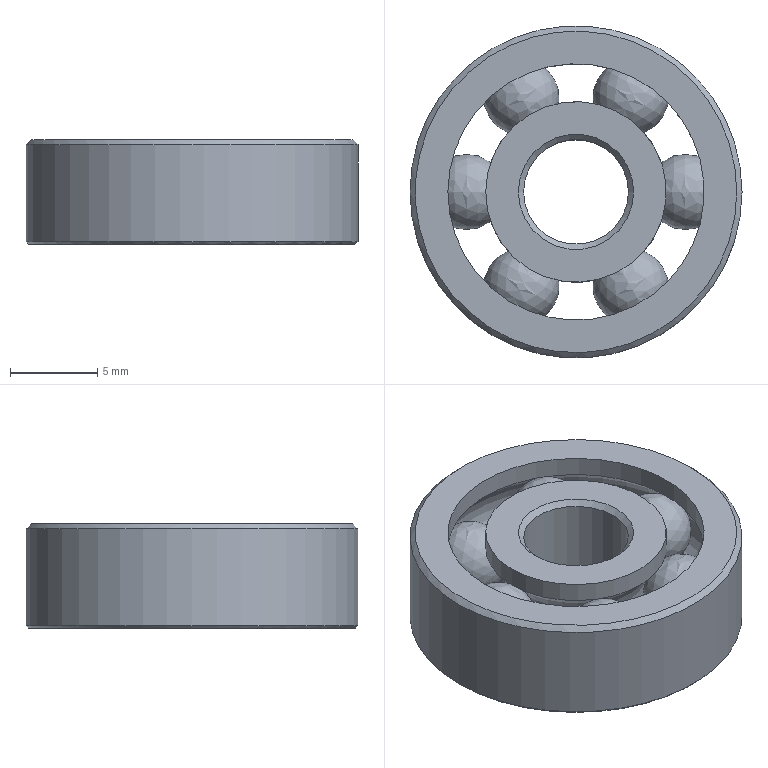Part | NX | features SWP104 11, INSTANCE_SET 5, CHAMFER 3, SKETCH 3, DATUM_CSYS 2, FSET 2, CIRCULAR_PATTERN 1, LINE 1 | 8 solids | 22 faces | box 19 x 19 x 6 mm | volume 1034 mm3 | sphere 6 | cylinder 5 | cone 5 | plane 4 | torus 2 | commonest cylinder face diameters 10.334 x2 6 x1 14.666 x1 19 x1
STEP:
#1=CARTESIAN_POINT('',(-2.042,-3.537,3.));
#2=VERTEX_POINT('',#1);
#3=VERTEX_LOOP('',#2);
#4=FACE_BOUND('',#3,.T.);
#5=CARTESIAN_POINT('',(-3.125,-5.413,3.));
#6=DIRECTION('',(-0.5,-0.866,0.));
#7=DIRECTION('',(0.,0.,1.));
#8=AXIS2_PLACEMENT_3D('',#5,#6,#7);
#9=SPHERICAL_SURFACE('',#8,2.166);
#10=ADVANCED_FACE('',(#4),#9,.T.);
#11=CLOSED_SHELL('',(#10));
#12=MANIFOLD_SOLID_BREP('',#11);
#13=CARTESIAN_POINT('',(5.167,0.,1.124));
#14=VERTEX_POINT('',#13);
#15=CARTESIAN_POINT('',(0.,0.,1.124));
#16=DIRECTION('',(0.,0.,1.));
#17=DIRECTION('',(1.,0.,0.));
#18=AXIS2_PLACEMENT_3D('',#15,#16,#17);
#19=CIRCLE('',#18,5.167);
#20=EDGE_CURVE('',#14,#14,#19,.T.);
#21=ORIENTED_EDGE('',*,*,#20,.F.);
#22=EDGE_LOOP('',(#21));
#23=FACE_BOUND('',#22,.T.);
#24=CARTESIAN_POINT('',(-5.167,0.,0.));
#25=VERTEX_POINT('',#24);
#26=CARTESIAN_POINT('',(0.,0.,0.));
#27=DIRECTION('',(0.,0.,-1.));
#28=DIRECTION('',(-1.,0.,0.));
#29=AXIS2_PLACEMENT_3D('',#26,#27,#28);
#30=CIRCLE('',#29,5.167);
#31=EDGE_CURVE('',#25,#25,#30,.T.);
#32=ORIENTED_EDGE('',*,*,#31,.F.);
#33=EDGE_LOOP('',(#32));
#34=FACE_BOUND('',#33,.T.);
#35=CARTESIAN_POINT('',(0.,0.,0.));
#36=DIRECTION('',(0.,0.,-1.));
#37=DIRECTION('',(-1.,0.,0.));
#38=AXIS2_PLACEMENT_3D('',#35,#36,#37);
#39=CYLINDRICAL_SURFACE('',#38,5.167);
#40=ADVANCED_FACE('',(#23,#34),#39,.T.);
#41=CARTESIAN_POINT('',(-3.,0.,0.3));
#42=VERTEX_POINT('',#41);
#43=CARTESIAN_POINT('',(0.,0.,0.3));
#44=DIRECTION('',(0.,0.,-1.));
#45=DIRECTION('',(-1.,0.,0.));
#46=AXIS2_PLACEMENT_3D('',#43,#44,#45);
#47=CIRCLE('',#46,3.);
#48=EDGE_CURVE('',#42,#42,#47,.T.);
#49=ORIENTED_EDGE('',*,*,#48,.T.);
#50=EDGE_LOOP('',(#49));
#51=FACE_BOUND('',#50,.T.);
#52=CARTESIAN_POINT('',(3.,0.,5.7));
#53=VERTEX_POINT('',#52);
#54=CARTESIAN_POINT('',(0.,0.,5.7));
#55=DIRECTION('',(0.,0.,1.));
#56=DIRECTION('',(1.,0.,0.));
#57=AXIS2_PLACEMENT_3D('',#54,#55,#56);
#58=CIRCLE('',#57,3.);
#59=EDGE_CURVE('',#53,#53,#58,.T.);
#60=ORIENTED_EDGE('',*,*,#59,.T.);
#61=EDGE_LOOP('',(#60));
#62=FACE_BOUND('',#61,.T.);
#63=CARTESIAN_POINT('',(0.,0.,0.));
#64=DIRECTION('',(0.,0.,-1.));
#65=DIRECTION('',(-1.,0.,0.));
#66=AXIS2_PLACEMENT_3D('',#63,#64,#65);
#67=CYLINDRICAL_SURFACE('',#66,3.);
#68=ADVANCED_FACE('',(#51,#62),#67,.F.);
#69=CARTESIAN_POINT('',(-3.3,0.,0.));
#70=VERTEX_POINT('',#69);
#71=CARTESIAN_POINT('',(0.,0.,0.));
#72=DIRECTION('',(0.,0.,-1.));
#73=DIRECTION('',(-1.,0.,0.));
#74=AXIS2_PLACEMENT_3D('',#71,#72,#73);
#75=CIRCLE('',#74,3.3);
#76=EDGE_CURVE('',#70,#70,#75,.F.);
#77=ORIENTED_EDGE('',*,*,#76,.T.);
#78=EDGE_LOOP('',(#77));
#79=FACE_BOUND('',#78,.T.);
#80=ORIENTED_EDGE('',*,*,#31,.T.);
#81=EDGE_LOOP('',(#80));
#82=FACE_BOUND('',#81,.T.);
#83=CARTESIAN_POINT('',(3.,0.,0.));
#84=DIRECTION('',(0.,0.,-1.));
#85=DIRECTION('',(-1.,0.,0.));
#86=AXIS2_PLACEMENT_3D('',#83,#84,#85);
#87=PLANE('',#86);
#88=ADVANCED_FACE('',(#79,#82),#87,.T.);
#89=CARTESIAN_POINT('',(-5.167,0.,4.876));
#90=VERTEX_POINT('',#89);
#91=CARTESIAN_POINT('',(0.,0.,4.876));
#92=DIRECTION('',(0.,0.,-1.));
#93=DIRECTION('',(-1.,0.,0.));
#94=AXIS2_PLACEMENT_3D('',#91,#92,#93);
#95=CIRCLE('',#94,5.167);
#96=EDGE_CURVE('',#90,#90,#95,.T.);
#97=ORIENTED_EDGE('',*,*,#96,.F.);
#98=EDGE_LOOP('',(#97));
#99=FACE_BOUND('',#98,.T.);
#100=CARTESIAN_POINT('',(-5.167,0.,6.));
#101=VERTEX_POINT('',#100);
#102=CARTESIAN_POINT('',(0.,0.,6.));
#103=DIRECTION('',(0.,0.,-1.));
#104=DIRECTION('',(-1.,0.,0.));
#105=AXIS2_PLACEMENT_3D('',#102,#103,#104);
#106=CIRCLE('',#105,5.167);
#107=EDGE_CURVE('',#101,#101,#106,.T.);
#108=ORIENTED_EDGE('',*,*,#107,.T.);
#109=EDGE_LOOP('',(#108));
#110=FACE_BOUND('',#109,.T.);
#111=CARTESIAN_POINT('',(0.,0.,0.));
#112=DIRECTION('',(0.,0.,-1.));
#113=DIRECTION('',(-1.,0.,0.));
#114=AXIS2_PLACEMENT_3D('',#111,#112,#113);
#115=CYLINDRICAL_SURFACE('',#114,5.167);
#116=ADVANCED_FACE('',(#99,#110),#115,.T.);
#117=CARTESIAN_POINT('',(3.3,0.,6.));
#118=VERTEX_POINT('',#117);
#119=CARTESIAN_POINT('',(0.,0.,6.));
#120=DIRECTION('',(0.,0.,1.));
#121=DIRECTION('',(1.,0.,0.));
#122=AXIS2_PLACEMENT_3D('',#119,#120,#121);
#123=CIRCLE('',#122,3.3);
#124=EDGE_CURVE('',#118,#118,#123,.F.);
#125=ORIENTED_EDGE('',*,*,#124,.T.);
#126=EDGE_LOOP('',(#125));
#127=FACE_BOUND('',#126,.T.);
#128=ORIENTED_EDGE('',*,*,#107,.F.);
#129=EDGE_LOOP('',(#128));
#130=FACE_BOUND('',#129,.T.);
#131=CARTESIAN_POINT('',(5.167,0.,6.));
#132=DIRECTION('',(0.,0.,1.));
#133=DIRECTION('',(1.,0.,0.));
#134=AXIS2_PLACEMENT_3D('',#131,#132,#133);
#135=PLANE('',#134);
#136=ADVANCED_FACE('',(#127,#130),#135,.T.);
#137=ORIENTED_EDGE('',*,*,#20,.T.);
#138=EDGE_LOOP('',(#137));
#139=FACE_BOUND('',#138,.T.);
#140=ORIENTED_EDGE('',*,*,#96,.T.);
#141=EDGE_LOOP('',(#140));
#142=FACE_BOUND('',#141,.T.);
#143=CARTESIAN_POINT('',(0.,0.,3.));
#144=DIRECTION('',(0.,0.,-1.));
#145=DIRECTION('',(-1.,0.,0.));
#146=AXIS2_PLACEMENT_3D('',#143,#144,#145);
#147=TOROIDAL_SURFACE('',#146,6.25,2.166);
#148=ADVANCED_FACE('',(#139,#142),#147,.F.);
#149=ORIENTED_EDGE('',*,*,#76,.F.);
#150=EDGE_LOOP('',(#149));
#151=FACE_BOUND('',#150,.T.);
#152=ORIENTED_EDGE('',*,*,#48,.F.);
#153=EDGE_LOOP('',(#152));
#154=FACE_BOUND('',#153,.T.);
#155=CARTESIAN_POINT('',(0.,0.,0.3));
#156=DIRECTION('',(0.,0.,-1.));
#157=DIRECTION('',(-1.,0.,0.));
#158=AXIS2_PLACEMENT_3D('',#155,#156,#157);
#159=CONICAL_SURFACE('',#158,3.,0.7854);
#160=ADVANCED_FACE('',(#151,#154),#159,.F.);
#161=ORIENTED_EDGE('',*,*,#59,.F.);
#162=EDGE_LOOP('',(#161));
#163=FACE_BOUND('',#162,.T.);
#164=ORIENTED_EDGE('',*,*,#124,.F.);
#165=EDGE_LOOP('',(#164));
#166=FACE_BOUND('',#165,.T.);
#167=CARTESIAN_POINT('',(0.,0.,6.));
#168=DIRECTION('',(0.,0.,1.));
#169=DIRECTION('',(1.,0.,0.));
#170=AXIS2_PLACEMENT_3D('',#167,#168,#169);
#171=CONICAL_SURFACE('',#170,3.3,0.7854);
#172=ADVANCED_FACE('',(#163,#166),#171,.F.);
#173=CLOSED_SHELL('',(#40,#68,#88,#116,#136,#148,#160,#172));
#174=MANIFOLD_SOLID_BREP('',#173);
#175=CARTESIAN_POINT('',(2.042,-3.537,3.));
#176=VERTEX_POINT('',#175);
#177=VERTEX_LOOP('',#176);
#178=FACE_BOUND('',#177,.T.);
#179=CARTESIAN_POINT('',(3.125,-5.413,3.));
#180=DIRECTION('',(0.5,-0.866,0.));
#181=DIRECTION('',(0.,0.,1.));
#182=AXIS2_PLACEMENT_3D('',#179,#180,#181);
#183=SPHERICAL_SURFACE('',#182,2.166);
#184=ADVANCED_FACE('',(#178),#183,.T.);
#185=CLOSED_SHELL('',(#184));
#186=MANIFOLD_SOLID_BREP('',#185);
#187=CARTESIAN_POINT('',(-9.5,0.,0.15));
#188=VERTEX_POINT('',#187);
#189=CARTESIAN_POINT('',(0.,0.,0.15));
#190=DIRECTION('',(0.,0.,-1.));
#191=DIRECTION('',(-1.,0.,0.));
#192=AXIS2_PLACEMENT_3D('',#189,#190,#191);
#193=CIRCLE('',#192,9.5);
#194=EDGE_CURVE('',#188,#188,#193,.F.);
#195=ORIENTED_EDGE('',*,*,#194,.T.);
#196=EDGE_LOOP('',(#195));
#197=FACE_BOUND('',#196,.T.);
#198=CARTESIAN_POINT('',(9.5,0.,5.7));
#199=VERTEX_POINT('',#198);
#200=CARTESIAN_POINT('',(0.,0.,5.7));
#201=DIRECTION('',(0.,0.,1.));
#202=DIRECTION('',(1.,0.,0.));
#203=AXIS2_PLACEMENT_3D('',#200,#201,#202);
#204=CIRCLE('',#203,9.5);
#205=EDGE_CURVE('',#199,#199,#204,.F.);
#206=ORIENTED_EDGE('',*,*,#205,.T.);
#207=EDGE_LOOP('',(#206));
#208=FACE_BOUND('',#207,.T.);
#209=CARTESIAN_POINT('',(0.,0.,0.));
#210=DIRECTION('',(0.,0.,-1.));
#211=DIRECTION('',(-1.,0.,0.));
#212=AXIS2_PLACEMENT_3D('',#209,#210,#211);
#213=CYLINDRICAL_SURFACE('',#212,9.5);
#214=ADVANCED_FACE('',(#197,#208),#213,.T.);
#215=CARTESIAN_POINT('',(9.2,0.,6.));
#216=VERTEX_POINT('',#215);
#217=CARTESIAN_POINT('',(0.,0.,6.));
#218=DIRECTION('',(0.,0.,1.));
#219=DIRECTION('',(1.,0.,0.));
#220=AXIS2_PLACEMENT_3D('',#217,#218,#219);
#221=CIRCLE('',#220,9.2);
#222=EDGE_CURVE('',#216,#216,#221,.T.);
#223=ORIENTED_EDGE('',*,*,#222,.T.);
#224=EDGE_LOOP('',(#223));
#225=FACE_BOUND('',#224,.T.);
#226=CARTESIAN_POINT('',(-7.333,0.,6.));
#227=VERTEX_POINT('',#226);
#228=CARTESIAN_POINT('',(0.,0.,6.));
#229=DIRECTION('',(0.,0.,-1.));
#230=DIRECTION('',(-1.,0.,0.));
#231=AXIS2_PLACEMENT_3D('',#228,#229,#230);
#232=CIRCLE('',#231,7.333);
#233=EDGE_CURVE('',#227,#227,#232,.T.);
#234=ORIENTED_EDGE('',*,*,#233,.T.);
#235=EDGE_LOOP('',(#234));
#236=FACE_BOUND('',#235,.T.);
#237=CARTESIAN_POINT('',(9.5,0.,6.));
#238=DIRECTION('',(0.,0.,1.));
#239=DIRECTION('',(1.,0.,0.));
#240=AXIS2_PLACEMENT_3D('',#237,#238,#239);
#241=PLANE('',#240);
#242=ADVANCED_FACE('',(#225,#236),#241,.T.);
#243=CARTESIAN_POINT('',(-7.333,0.,4.876));
#244=VERTEX_POINT('',#243);
#245=CARTESIAN_POINT('',(0.,0.,4.876));
#246=DIRECTION('',(0.,0.,-1.));
#247=DIRECTION('',(-1.,0.,0.));
#248=AXIS2_PLACEMENT_3D('',#245,#246,#247);
#249=CIRCLE('',#248,7.333);
#250=EDGE_CURVE('',#244,#244,#249,.F.);
#251=ORIENTED_EDGE('',*,*,#250,.F.);
#252=EDGE_LOOP('',(#251));
#253=FACE_BOUND('',#252,.T.);
#254=ORIENTED_EDGE('',*,*,#233,.F.);
#255=EDGE_LOOP('',(#254));
#256=FACE_BOUND('',#255,.T.);
#257=CARTESIAN_POINT('',(0.,0.,0.));
#258=DIRECTION('',(0.,0.,-1.));
#259=DIRECTION('',(-1.,0.,0.));
#260=AXIS2_PLACEMENT_3D('',#257,#258,#259);
#261=CYLINDRICAL_SURFACE('',#260,7.333);
#262=ADVANCED_FACE('',(#253,#256),#261,.F.);
#263=CARTESIAN_POINT('',(-9.35,0.,0.));
#264=VERTEX_POINT('',#263);
#265=CARTESIAN_POINT('',(0.,0.,0.));
#266=DIRECTION('',(0.,0.,-1.));
#267=DIRECTION('',(-1.,0.,0.));
#268=AXIS2_PLACEMENT_3D('',#265,#266,#267);
#269=CIRCLE('',#268,9.35);
#270=EDGE_CURVE('',#264,#264,#269,.T.);
#271=ORIENTED_EDGE('',*,*,#270,.T.);
#272=EDGE_LOOP('',(#271));
#273=FACE_BOUND('',#272,.T.);
#274=CARTESIAN_POINT('',(-7.766,0.,0.));
#275=VERTEX_POINT('',#274);
#276=CARTESIAN_POINT('',(0.,0.,0.));
#277=DIRECTION('',(0.,0.,-1.));
#278=DIRECTION('',(-1.,0.,0.));
#279=AXIS2_PLACEMENT_3D('',#276,#277,#278);
#280=CIRCLE('',#279,7.766);
#281=EDGE_CURVE('',#275,#275,#280,.T.);
#282=ORIENTED_EDGE('',*,*,#281,.F.);
#283=EDGE_LOOP('',(#282));
#284=FACE_BOUND('',#283,.T.);
#285=CARTESIAN_POINT('',(7.333,0.,0.));
#286=DIRECTION('',(0.,0.,-1.));
#287=DIRECTION('',(-1.,0.,0.));
#288=AXIS2_PLACEMENT_3D('',#285,#286,#287);
#289=PLANE('',#288);
#290=ADVANCED_FACE('',(#273,#284),#289,.T.);
#291=CARTESIAN_POINT('',(-7.333,0.,1.124));
#292=VERTEX_POINT('',#291);
#293=CARTESIAN_POINT('',(0.,0.,1.124));
#294=DIRECTION('',(0.,0.,-1.));
#295=DIRECTION('',(-1.,0.,0.));
#296=AXIS2_PLACEMENT_3D('',#293,#294,#295);
#297=CIRCLE('',#296,7.333);
#298=EDGE_CURVE('',#292,#292,#297,.T.);
#299=ORIENTED_EDGE('',*,*,#298,.T.);
#300=EDGE_LOOP('',(#299));
#301=FACE_BOUND('',#300,.T.);
#302=ORIENTED_EDGE('',*,*,#250,.T.);
#303=EDGE_LOOP('',(#302));
#304=FACE_BOUND('',#303,.T.);
#305=CARTESIAN_POINT('',(0.,0.,3.));
#306=DIRECTION('',(0.,0.,-1.));
#307=DIRECTION('',(-1.,0.,0.));
#308=AXIS2_PLACEMENT_3D('',#305,#306,#307);
#309=TOROIDAL_SURFACE('',#308,6.25,2.166);
#310=ADVANCED_FACE('',(#301,#304),#309,.F.);
#311=ORIENTED_EDGE('',*,*,#298,.F.);
#312=EDGE_LOOP('',(#311));
#313=FACE_BOUND('',#312,.T.);
#314=ORIENTED_EDGE('',*,*,#281,.T.);
#315=EDGE_LOOP('',(#314));
#316=FACE_BOUND('',#315,.T.);
#317=CARTESIAN_POINT('',(0.,0.,0.));
#318=DIRECTION('',(0.,0.,-1.));
#319=DIRECTION('',(-1.,0.,0.));
#320=AXIS2_PLACEMENT_3D('',#317,#318,#319);
#321=CONICAL_SURFACE('',#320,7.766,0.368);
#322=ADVANCED_FACE('',(#313,#316),#321,.F.);
#323=ORIENTED_EDGE('',*,*,#222,.F.);
#324=EDGE_LOOP('',(#323));
#325=FACE_BOUND('',#324,.T.);
#326=ORIENTED_EDGE('',*,*,#205,.F.);
#327=EDGE_LOOP('',(#326));
#328=FACE_BOUND('',#327,.T.);
#329=CARTESIAN_POINT('',(0.,0.,5.7));
#330=DIRECTION('',(0.,0.,-1.));
#331=DIRECTION('',(-1.,0.,0.));
#332=AXIS2_PLACEMENT_3D('',#329,#330,#331);
#333=CONICAL_SURFACE('',#332,9.5,0.7854);
#334=ADVANCED_FACE('',(#325,#328),#333,.T.);
#335=ORIENTED_EDGE('',*,*,#194,.F.);
#336=EDGE_LOOP('',(#335));
#337=FACE_BOUND('',#336,.T.);
#338=ORIENTED_EDGE('',*,*,#270,.F.);
#339=EDGE_LOOP('',(#338));
#340=FACE_BOUND('',#339,.T.);
#341=CARTESIAN_POINT('',(0.,0.,0.));
#342=DIRECTION('',(0.,0.,1.));
#343=DIRECTION('',(1.,0.,0.));
#344=AXIS2_PLACEMENT_3D('',#341,#342,#343);
#345=CONICAL_SURFACE('',#344,9.35,0.7854);
#346=ADVANCED_FACE('',(#337,#340),#345,.T.);
#347=CLOSED_SHELL('',(#214,#242,#262,#290,#310,#322,#334,#346));
#348=MANIFOLD_SOLID_BREP('',#347);
#349=CARTESIAN_POINT('',(4.084,0.,3.));
#350=VERTEX_POINT('',#349);
#351=VERTEX_LOOP('',#350);
#352=FACE_BOUND('',#351,.T.);
#353=CARTESIAN_POINT('',(6.25,0.,3.));
#354=DIRECTION('',(1.,0.,0.));
#355=DIRECTION('',(0.,0.,1.));
#356=AXIS2_PLACEMENT_3D('',#353,#354,#355);
#357=SPHERICAL_SURFACE('',#356,2.166);
#358=ADVANCED_FACE('',(#352),#357,.T.);
#359=CLOSED_SHELL('',(#358));
#360=MANIFOLD_SOLID_BREP('',#359);
#361=CARTESIAN_POINT('',(-4.084,0.,3.));
#362=VERTEX_POINT('',#361);
#363=VERTEX_LOOP('',#362);
#364=FACE_BOUND('',#363,.T.);
#365=CARTESIAN_POINT('',(-6.25,0.,3.));
#366=DIRECTION('',(-1.,0.,0.));
#367=DIRECTION('',(0.,0.,1.));
#368=AXIS2_PLACEMENT_3D('',#365,#366,#367);
#369=SPHERICAL_SURFACE('',#368,2.166);
#370=ADVANCED_FACE('',(#364),#369,.T.);
#371=CLOSED_SHELL('',(#370));
#372=MANIFOLD_SOLID_BREP('',#371);
#373=CARTESIAN_POINT('',(-2.042,3.537,3.));
#374=VERTEX_POINT('',#373);
#375=VERTEX_LOOP('',#374);
#376=FACE_BOUND('',#375,.T.);
#377=CARTESIAN_POINT('',(-3.125,5.413,3.));
#378=DIRECTION('',(-0.5,0.866,0.));
#379=DIRECTION('',(0.,0.,1.));
#380=AXIS2_PLACEMENT_3D('',#377,#378,#379);
#381=SPHERICAL_SURFACE('',#380,2.166);
#382=ADVANCED_FACE('',(#376),#381,.T.);
#383=CLOSED_SHELL('',(#382));
#384=MANIFOLD_SOLID_BREP('',#383);
#385=CARTESIAN_POINT('',(2.042,3.537,3.));
#386=VERTEX_POINT('',#385);
#387=VERTEX_LOOP('',#386);
#388=FACE_BOUND('',#387,.T.);
#389=CARTESIAN_POINT('',(3.125,5.413,3.));
#390=DIRECTION('',(0.5,0.866,0.));
#391=DIRECTION('',(0.,0.,1.));
#392=AXIS2_PLACEMENT_3D('',#389,#390,#391);
#393=SPHERICAL_SURFACE('',#392,2.166);
#394=ADVANCED_FACE('',(#388),#393,.T.);
#395=CLOSED_SHELL('',(#394));
#396=MANIFOLD_SOLID_BREP('',#395);
#397=(LENGTH_UNIT()NAMED_UNIT(*)SI_UNIT(.MILLI.,.METRE.));
#398=UNCERTAINTY_MEASURE_WITH_UNIT(LENGTH_MEASURE(0.00001),#397,'','');
#399=(NAMED_UNIT(*)PLANE_ANGLE_UNIT()SI_UNIT($,.RADIAN.));
#400=(NAMED_UNIT(*)SI_UNIT($,.STERADIAN.)SOLID_ANGLE_UNIT());
#401=(GEOMETRIC_REPRESENTATION_CONTEXT(3)GLOBAL_UNCERTAINTY_ASSIGNED_CONTEXT((#398))GLOBAL_UNIT_ASSIGNED_CONTEXT((#397,#399,#400))REPRESENTATION_CONTEXT('',''));
#402=ADVANCED_BREP_SHAPE_REPRESENTATION('',(#12,#174,#186,#348,#360,#372,#384,#396),#401);